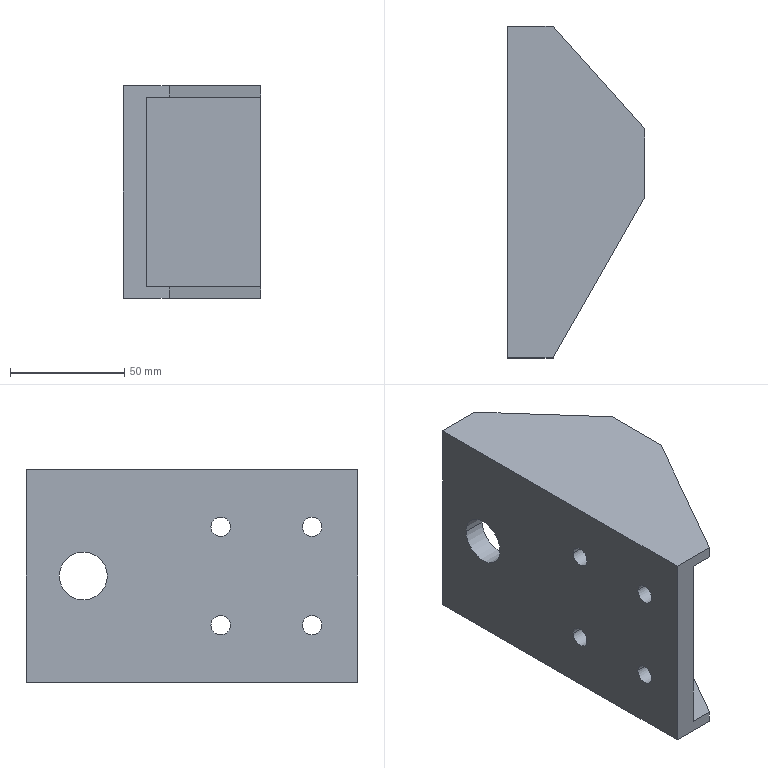Part | NX | features BREP 1 | 1 solid | 28 faces | box 60 x 145 x 93 mm | volume 220117 mm3 | plane 18 | cylinder 10 | commonest cylinder face diameters 8.5 x8 21 x2
STEP:
#1=CARTESIAN_POINT('',(-5.,58.,0.));
#2=VERTEX_POINT('',#1);
#3=CARTESIAN_POINT('',(-5.,37.,0.));
#4=VERTEX_POINT('',#3);
#5=CARTESIAN_POINT('',(-5.,47.5,0.));
#6=DIRECTION('',(-1.,0.,0.));
#7=DIRECTION('',(0.,1.,0.));
#8=AXIS2_PLACEMENT_3D('',#5,#6,#7);
#9=CIRCLE('',#8,10.5);
#10=EDGE_CURVE('',#2,#4,#9,.T.);
#11=ORIENTED_EDGE('',*,*,#10,.T.);
#12=CARTESIAN_POINT('',(5.,37.,0.));
#13=VERTEX_POINT('',#12);
#14=CARTESIAN_POINT('',(-5.,37.,0.));
#15=DIRECTION('',(1.,0.,0.));
#16=VECTOR('',#15,1000.);
#17=LINE('',#14,#16);
#18=EDGE_CURVE('',#13,#4,#17,.F.);
#19=ORIENTED_EDGE('',*,*,#18,.F.);
#20=CARTESIAN_POINT('',(5.,58.,0.));
#21=VERTEX_POINT('',#20);
#22=CARTESIAN_POINT('',(5.,47.5,0.));
#23=DIRECTION('',(-1.,0.,0.));
#24=DIRECTION('',(0.,1.,0.));
#25=AXIS2_PLACEMENT_3D('',#22,#23,#24);
#26=CIRCLE('',#25,10.5);
#27=EDGE_CURVE('',#21,#13,#26,.T.);
#28=ORIENTED_EDGE('',*,*,#27,.F.);
#29=CARTESIAN_POINT('',(-5.,58.,0.));
#30=DIRECTION('',(1.,0.,0.));
#31=VECTOR('',#30,1000.);
#32=LINE('',#29,#31);
#33=EDGE_CURVE('',#21,#2,#32,.F.);
#34=ORIENTED_EDGE('',*,*,#33,.T.);
#35=EDGE_LOOP('',(#11,#19,#28,#34));
#36=FACE_BOUND('',#35,.T.);
#37=CARTESIAN_POINT('',(-5.,47.5,0.));
#38=DIRECTION('',(1.,0.,0.));
#39=DIRECTION('',(0.,1.,0.));
#40=AXIS2_PLACEMENT_3D('',#37,#38,#39);
#41=CYLINDRICAL_SURFACE('',#40,10.5);
#42=ADVANCED_FACE('',(#36),#41,.F.);
#43=CARTESIAN_POINT('',(-5.,-8.25,21.5));
#44=VERTEX_POINT('',#43);
#45=CARTESIAN_POINT('',(-5.,-16.75,21.5));
#46=VERTEX_POINT('',#45);
#47=CARTESIAN_POINT('',(-5.,-12.5,21.5));
#48=DIRECTION('',(-1.,0.,0.));
#49=DIRECTION('',(0.,1.,0.));
#50=AXIS2_PLACEMENT_3D('',#47,#48,#49);
#51=CIRCLE('',#50,4.25);
#52=EDGE_CURVE('',#44,#46,#51,.T.);
#53=ORIENTED_EDGE('',*,*,#52,.T.);
#54=CARTESIAN_POINT('',(5.,-16.75,21.5));
#55=VERTEX_POINT('',#54);
#56=CARTESIAN_POINT('',(-5.,-16.75,21.5));
#57=DIRECTION('',(1.,0.,0.));
#58=VECTOR('',#57,1000.);
#59=LINE('',#56,#58);
#60=EDGE_CURVE('',#55,#46,#59,.F.);
#61=ORIENTED_EDGE('',*,*,#60,.F.);
#62=CARTESIAN_POINT('',(5.,-8.25,21.5));
#63=VERTEX_POINT('',#62);
#64=CARTESIAN_POINT('',(5.,-12.5,21.5));
#65=DIRECTION('',(-1.,0.,0.));
#66=DIRECTION('',(0.,1.,0.));
#67=AXIS2_PLACEMENT_3D('',#64,#65,#66);
#68=CIRCLE('',#67,4.25);
#69=EDGE_CURVE('',#63,#55,#68,.T.);
#70=ORIENTED_EDGE('',*,*,#69,.F.);
#71=CARTESIAN_POINT('',(-5.,-8.25,21.5));
#72=DIRECTION('',(1.,0.,0.));
#73=VECTOR('',#72,1000.);
#74=LINE('',#71,#73);
#75=EDGE_CURVE('',#63,#44,#74,.F.);
#76=ORIENTED_EDGE('',*,*,#75,.T.);
#77=EDGE_LOOP('',(#53,#61,#70,#76));
#78=FACE_BOUND('',#77,.T.);
#79=CARTESIAN_POINT('',(-5.,-12.5,21.5));
#80=DIRECTION('',(1.,0.,0.));
#81=DIRECTION('',(0.,1.,0.));
#82=AXIS2_PLACEMENT_3D('',#79,#80,#81);
#83=CYLINDRICAL_SURFACE('',#82,4.25);
#84=ADVANCED_FACE('',(#78),#83,.F.);
#85=CARTESIAN_POINT('',(-5.,-8.25,-21.5));
#86=VERTEX_POINT('',#85);
#87=CARTESIAN_POINT('',(-5.,-16.75,-21.5));
#88=VERTEX_POINT('',#87);
#89=CARTESIAN_POINT('',(-5.,-12.5,-21.5));
#90=DIRECTION('',(-1.,0.,0.));
#91=DIRECTION('',(0.,1.,0.));
#92=AXIS2_PLACEMENT_3D('',#89,#90,#91);
#93=CIRCLE('',#92,4.25);
#94=EDGE_CURVE('',#86,#88,#93,.T.);
#95=ORIENTED_EDGE('',*,*,#94,.T.);
#96=CARTESIAN_POINT('',(5.,-16.75,-21.5));
#97=VERTEX_POINT('',#96);
#98=CARTESIAN_POINT('',(-5.,-16.75,-21.5));
#99=DIRECTION('',(1.,0.,0.));
#100=VECTOR('',#99,1000.);
#101=LINE('',#98,#100);
#102=EDGE_CURVE('',#97,#88,#101,.F.);
#103=ORIENTED_EDGE('',*,*,#102,.F.);
#104=CARTESIAN_POINT('',(5.,-8.25,-21.5));
#105=VERTEX_POINT('',#104);
#106=CARTESIAN_POINT('',(5.,-12.5,-21.5));
#107=DIRECTION('',(-1.,0.,0.));
#108=DIRECTION('',(0.,1.,0.));
#109=AXIS2_PLACEMENT_3D('',#106,#107,#108);
#110=CIRCLE('',#109,4.25);
#111=EDGE_CURVE('',#105,#97,#110,.T.);
#112=ORIENTED_EDGE('',*,*,#111,.F.);
#113=CARTESIAN_POINT('',(-5.,-8.25,-21.5));
#114=DIRECTION('',(1.,0.,0.));
#115=VECTOR('',#114,1000.);
#116=LINE('',#113,#115);
#117=EDGE_CURVE('',#105,#86,#116,.F.);
#118=ORIENTED_EDGE('',*,*,#117,.T.);
#119=EDGE_LOOP('',(#95,#103,#112,#118));
#120=FACE_BOUND('',#119,.T.);
#121=CARTESIAN_POINT('',(-5.,-12.5,-21.5));
#122=DIRECTION('',(1.,0.,0.));
#123=DIRECTION('',(0.,1.,0.));
#124=AXIS2_PLACEMENT_3D('',#121,#122,#123);
#125=CYLINDRICAL_SURFACE('',#124,4.25);
#126=ADVANCED_FACE('',(#120),#125,.F.);
#127=CARTESIAN_POINT('',(-5.,-48.25,-21.5));
#128=VERTEX_POINT('',#127);
#129=CARTESIAN_POINT('',(-5.,-56.75,-21.5));
#130=VERTEX_POINT('',#129);
#131=CARTESIAN_POINT('',(-5.,-52.5,-21.5));
#132=DIRECTION('',(-1.,0.,0.));
#133=DIRECTION('',(0.,1.,0.));
#134=AXIS2_PLACEMENT_3D('',#131,#132,#133);
#135=CIRCLE('',#134,4.25);
#136=EDGE_CURVE('',#128,#130,#135,.T.);
#137=ORIENTED_EDGE('',*,*,#136,.T.);
#138=CARTESIAN_POINT('',(5.,-56.75,-21.5));
#139=VERTEX_POINT('',#138);
#140=CARTESIAN_POINT('',(-5.,-56.75,-21.5));
#141=DIRECTION('',(1.,0.,0.));
#142=VECTOR('',#141,1000.);
#143=LINE('',#140,#142);
#144=EDGE_CURVE('',#139,#130,#143,.F.);
#145=ORIENTED_EDGE('',*,*,#144,.F.);
#146=CARTESIAN_POINT('',(5.,-48.25,-21.5));
#147=VERTEX_POINT('',#146);
#148=CARTESIAN_POINT('',(5.,-52.5,-21.5));
#149=DIRECTION('',(-1.,0.,0.));
#150=DIRECTION('',(0.,1.,0.));
#151=AXIS2_PLACEMENT_3D('',#148,#149,#150);
#152=CIRCLE('',#151,4.25);
#153=EDGE_CURVE('',#147,#139,#152,.T.);
#154=ORIENTED_EDGE('',*,*,#153,.F.);
#155=CARTESIAN_POINT('',(-5.,-48.25,-21.5));
#156=DIRECTION('',(1.,0.,0.));
#157=VECTOR('',#156,1000.);
#158=LINE('',#155,#157);
#159=EDGE_CURVE('',#147,#128,#158,.F.);
#160=ORIENTED_EDGE('',*,*,#159,.T.);
#161=EDGE_LOOP('',(#137,#145,#154,#160));
#162=FACE_BOUND('',#161,.T.);
#163=CARTESIAN_POINT('',(-5.,-52.5,-21.5));
#164=DIRECTION('',(1.,0.,0.));
#165=DIRECTION('',(0.,1.,0.));
#166=AXIS2_PLACEMENT_3D('',#163,#164,#165);
#167=CYLINDRICAL_SURFACE('',#166,4.25);
#168=ADVANCED_FACE('',(#162),#167,.F.);
#169=CARTESIAN_POINT('',(-5.,-48.25,21.5));
#170=VERTEX_POINT('',#169);
#171=CARTESIAN_POINT('',(-5.,-56.75,21.5));
#172=VERTEX_POINT('',#171);
#173=CARTESIAN_POINT('',(-5.,-52.5,21.5));
#174=DIRECTION('',(-1.,0.,0.));
#175=DIRECTION('',(0.,1.,0.));
#176=AXIS2_PLACEMENT_3D('',#173,#174,#175);
#177=CIRCLE('',#176,4.25);
#178=EDGE_CURVE('',#170,#172,#177,.T.);
#179=ORIENTED_EDGE('',*,*,#178,.T.);
#180=CARTESIAN_POINT('',(5.,-56.75,21.5));
#181=VERTEX_POINT('',#180);
#182=CARTESIAN_POINT('',(-5.,-56.75,21.5));
#183=DIRECTION('',(1.,0.,0.));
#184=VECTOR('',#183,1000.);
#185=LINE('',#182,#184);
#186=EDGE_CURVE('',#181,#172,#185,.F.);
#187=ORIENTED_EDGE('',*,*,#186,.F.);
#188=CARTESIAN_POINT('',(5.,-48.25,21.5));
#189=VERTEX_POINT('',#188);
#190=CARTESIAN_POINT('',(5.,-52.5,21.5));
#191=DIRECTION('',(-1.,0.,0.));
#192=DIRECTION('',(0.,1.,0.));
#193=AXIS2_PLACEMENT_3D('',#190,#191,#192);
#194=CIRCLE('',#193,4.25);
#195=EDGE_CURVE('',#189,#181,#194,.T.);
#196=ORIENTED_EDGE('',*,*,#195,.F.);
#197=CARTESIAN_POINT('',(-5.,-48.25,21.5));
#198=DIRECTION('',(1.,0.,0.));
#199=VECTOR('',#198,1000.);
#200=LINE('',#197,#199);
#201=EDGE_CURVE('',#189,#170,#200,.F.);
#202=ORIENTED_EDGE('',*,*,#201,.T.);
#203=EDGE_LOOP('',(#179,#187,#196,#202));
#204=FACE_BOUND('',#203,.T.);
#205=CARTESIAN_POINT('',(-5.,-52.5,21.5));
#206=DIRECTION('',(1.,0.,0.));
#207=DIRECTION('',(0.,1.,0.));
#208=AXIS2_PLACEMENT_3D('',#205,#206,#207);
#209=CYLINDRICAL_SURFACE('',#208,4.25);
#210=ADVANCED_FACE('',(#204),#209,.F.);
#211=CARTESIAN_POINT('',(-5.,-72.5,46.5));
#212=VERTEX_POINT('',#211);
#213=CARTESIAN_POINT('',(-5.,-72.5,-46.5));
#214=VERTEX_POINT('',#213);
#215=CARTESIAN_POINT('',(-5.,-72.5,46.5));
#216=DIRECTION('',(0.,0.,-1.));
#217=VECTOR('',#216,1000.);
#218=LINE('',#215,#217);
#219=EDGE_CURVE('',#212,#214,#218,.T.);
#220=ORIENTED_EDGE('',*,*,#219,.F.);
#221=CARTESIAN_POINT('',(-5.,72.5,46.5));
#222=VERTEX_POINT('',#221);
#223=CARTESIAN_POINT('',(-5.,72.5,46.5));
#224=DIRECTION('',(0.,-1.,0.));
#225=VECTOR('',#224,1000.);
#226=LINE('',#223,#225);
#227=EDGE_CURVE('',#222,#212,#226,.T.);
#228=ORIENTED_EDGE('',*,*,#227,.F.);
#229=CARTESIAN_POINT('',(-5.,72.5,-46.5));
#230=VERTEX_POINT('',#229);
#231=CARTESIAN_POINT('',(-5.,72.5,46.5));
#232=DIRECTION('',(0.,0.,1.));
#233=VECTOR('',#232,1000.);
#234=LINE('',#231,#233);
#235=EDGE_CURVE('',#230,#222,#234,.T.);
#236=ORIENTED_EDGE('',*,*,#235,.F.);
#237=CARTESIAN_POINT('',(-5.,72.5,-46.5));
#238=DIRECTION('',(0.,1.,0.));
#239=VECTOR('',#238,1000.);
#240=LINE('',#237,#239);
#241=EDGE_CURVE('',#214,#230,#240,.T.);
#242=ORIENTED_EDGE('',*,*,#241,.F.);
#243=EDGE_LOOP('',(#220,#228,#236,#242));
#244=FACE_BOUND('',#243,.T.);
#245=ORIENTED_EDGE('',*,*,#10,.F.);
#246=CARTESIAN_POINT('',(-5.,47.5,0.));
#247=DIRECTION('',(-1.,0.,0.));
#248=DIRECTION('',(0.,1.,0.));
#249=AXIS2_PLACEMENT_3D('',#246,#247,#248);
#250=CIRCLE('',#249,10.5);
#251=EDGE_CURVE('',#4,#2,#250,.T.);
#252=ORIENTED_EDGE('',*,*,#251,.F.);
#253=EDGE_LOOP('',(#245,#252));
#254=FACE_BOUND('',#253,.T.);
#255=ORIENTED_EDGE('',*,*,#52,.F.);
#256=CARTESIAN_POINT('',(-5.,-12.5,21.5));
#257=DIRECTION('',(-1.,0.,0.));
#258=DIRECTION('',(0.,1.,0.));
#259=AXIS2_PLACEMENT_3D('',#256,#257,#258);
#260=CIRCLE('',#259,4.25);
#261=EDGE_CURVE('',#46,#44,#260,.T.);
#262=ORIENTED_EDGE('',*,*,#261,.F.);
#263=EDGE_LOOP('',(#255,#262));
#264=FACE_BOUND('',#263,.T.);
#265=ORIENTED_EDGE('',*,*,#94,.F.);
#266=CARTESIAN_POINT('',(-5.,-12.5,-21.5));
#267=DIRECTION('',(-1.,0.,0.));
#268=DIRECTION('',(0.,1.,0.));
#269=AXIS2_PLACEMENT_3D('',#266,#267,#268);
#270=CIRCLE('',#269,4.25);
#271=EDGE_CURVE('',#88,#86,#270,.T.);
#272=ORIENTED_EDGE('',*,*,#271,.F.);
#273=EDGE_LOOP('',(#265,#272));
#274=FACE_BOUND('',#273,.T.);
#275=ORIENTED_EDGE('',*,*,#136,.F.);
#276=CARTESIAN_POINT('',(-5.,-52.5,-21.5));
#277=DIRECTION('',(-1.,0.,0.));
#278=DIRECTION('',(0.,1.,0.));
#279=AXIS2_PLACEMENT_3D('',#276,#277,#278);
#280=CIRCLE('',#279,4.25);
#281=EDGE_CURVE('',#130,#128,#280,.T.);
#282=ORIENTED_EDGE('',*,*,#281,.F.);
#283=EDGE_LOOP('',(#275,#282));
#284=FACE_BOUND('',#283,.T.);
#285=ORIENTED_EDGE('',*,*,#178,.F.);
#286=CARTESIAN_POINT('',(-5.,-52.5,21.5));
#287=DIRECTION('',(-1.,0.,0.));
#288=DIRECTION('',(0.,1.,0.));
#289=AXIS2_PLACEMENT_3D('',#286,#287,#288);
#290=CIRCLE('',#289,4.25);
#291=EDGE_CURVE('',#172,#170,#290,.T.);
#292=ORIENTED_EDGE('',*,*,#291,.F.);
#293=EDGE_LOOP('',(#285,#292));
#294=FACE_BOUND('',#293,.T.);
#295=CARTESIAN_POINT('',(-5.,72.5,46.5));
#296=DIRECTION('',(1.,0.,0.));
#297=DIRECTION('',(0.,1.,0.));
#298=AXIS2_PLACEMENT_3D('',#295,#296,#297);
#299=PLANE('',#298);
#300=ADVANCED_FACE('',(#244,#254,#264,#274,#284,#294),#299,.F.);
#301=CARTESIAN_POINT('',(55.,-2.5,-46.5));
#302=VERTEX_POINT('',#301);
#303=CARTESIAN_POINT('',(55.,27.5,-46.5));
#304=VERTEX_POINT('',#303);
#305=CARTESIAN_POINT('',(55.,-72.5,-46.5));
#306=DIRECTION('',(0.,1.,0.));
#307=VECTOR('',#306,1000.);
#308=LINE('',#305,#307);
#309=EDGE_CURVE('',#302,#304,#308,.T.);
#310=ORIENTED_EDGE('',*,*,#309,.F.);
#311=CARTESIAN_POINT('',(15.,-72.5,-46.5));
#312=VERTEX_POINT('',#311);
#313=CARTESIAN_POINT('',(15.,-72.5,-46.5));
#314=DIRECTION('',(0.4961,0.8682,0.));
#315=VECTOR('',#314,1000.);
#316=LINE('',#313,#315);
#317=EDGE_CURVE('',#312,#302,#316,.T.);
#318=ORIENTED_EDGE('',*,*,#317,.F.);
#319=CARTESIAN_POINT('',(5.,-72.5,-46.5));
#320=DIRECTION('',(1.,0.,0.));
#321=VECTOR('',#320,1000.);
#322=LINE('',#319,#321);
#323=EDGE_CURVE('',#214,#312,#322,.T.);
#324=ORIENTED_EDGE('',*,*,#323,.F.);
#325=ORIENTED_EDGE('',*,*,#241,.T.);
#326=CARTESIAN_POINT('',(15.,72.5,-46.5));
#327=VERTEX_POINT('',#326);
#328=CARTESIAN_POINT('',(5.,72.5,-46.5));
#329=DIRECTION('',(-1.,0.,0.));
#330=VECTOR('',#329,1000.);
#331=LINE('',#328,#330);
#332=EDGE_CURVE('',#327,#230,#331,.T.);
#333=ORIENTED_EDGE('',*,*,#332,.F.);
#334=CARTESIAN_POINT('',(55.,27.5,-46.5));
#335=DIRECTION('',(-0.6644,0.7474,0.));
#336=VECTOR('',#335,1000.);
#337=LINE('',#334,#336);
#338=EDGE_CURVE('',#304,#327,#337,.T.);
#339=ORIENTED_EDGE('',*,*,#338,.F.);
#340=EDGE_LOOP('',(#310,#318,#324,#325,#333,#339));
#341=FACE_BOUND('',#340,.T.);
#342=CARTESIAN_POINT('',(5.,-72.5,-46.5));
#343=DIRECTION('',(0.,0.,1.));
#344=DIRECTION('',(1.,0.,0.));
#345=AXIS2_PLACEMENT_3D('',#342,#343,#344);
#346=PLANE('',#345);
#347=ADVANCED_FACE('',(#341),#346,.F.);
#348=CARTESIAN_POINT('',(15.,-72.5,-41.5));
#349=VERTEX_POINT('',#348);
#350=CARTESIAN_POINT('',(15.,-72.5,46.5));
#351=DIRECTION('',(0.,0.,-1.));
#352=VECTOR('',#351,1000.);
#353=LINE('',#350,#352);
#354=EDGE_CURVE('',#349,#312,#353,.T.);
#355=ORIENTED_EDGE('',*,*,#354,.F.);
#356=CARTESIAN_POINT('',(5.,-72.5,-41.5));
#357=VERTEX_POINT('',#356);
#358=CARTESIAN_POINT('',(-5.,-72.5,-41.5));
#359=DIRECTION('',(1.,0.,0.));
#360=VECTOR('',#359,1000.);
#361=LINE('',#358,#360);
#362=EDGE_CURVE('',#357,#349,#361,.T.);
#363=ORIENTED_EDGE('',*,*,#362,.F.);
#364=CARTESIAN_POINT('',(5.,-72.5,41.5));
#365=VERTEX_POINT('',#364);
#366=CARTESIAN_POINT('',(5.,-72.5,46.5));
#367=DIRECTION('',(0.,0.,-1.));
#368=VECTOR('',#367,1000.);
#369=LINE('',#366,#368);
#370=EDGE_CURVE('',#365,#357,#369,.T.);
#371=ORIENTED_EDGE('',*,*,#370,.F.);
#372=CARTESIAN_POINT('',(15.,-72.5,41.5));
#373=VERTEX_POINT('',#372);
#374=CARTESIAN_POINT('',(-5.,-72.5,41.5));
#375=DIRECTION('',(-1.,0.,0.));
#376=VECTOR('',#375,1000.);
#377=LINE('',#374,#376);
#378=EDGE_CURVE('',#373,#365,#377,.T.);
#379=ORIENTED_EDGE('',*,*,#378,.F.);
#380=CARTESIAN_POINT('',(15.,-72.5,46.5));
#381=VERTEX_POINT('',#380);
#382=CARTESIAN_POINT('',(15.,-72.5,46.5));
#383=DIRECTION('',(0.,0.,-1.));
#384=VECTOR('',#383,1000.);
#385=LINE('',#382,#384);
#386=EDGE_CURVE('',#381,#373,#385,.T.);
#387=ORIENTED_EDGE('',*,*,#386,.F.);
#388=CARTESIAN_POINT('',(-5.,-72.5,46.5));
#389=DIRECTION('',(1.,0.,0.));
#390=VECTOR('',#389,1000.);
#391=LINE('',#388,#390);
#392=EDGE_CURVE('',#212,#381,#391,.T.);
#393=ORIENTED_EDGE('',*,*,#392,.F.);
#394=ORIENTED_EDGE('',*,*,#219,.T.);
#395=ORIENTED_EDGE('',*,*,#323,.T.);
#396=EDGE_LOOP('',(#355,#363,#371,#379,#387,#393,#394,#395));
#397=FACE_BOUND('',#396,.T.);
#398=CARTESIAN_POINT('',(-5.,-72.5,46.5));
#399=DIRECTION('',(0.,1.,0.));
#400=DIRECTION('',(1.,0.,0.));
#401=AXIS2_PLACEMENT_3D('',#398,#399,#400);
#402=PLANE('',#401);
#403=ADVANCED_FACE('',(#397),#402,.F.);
#404=CARTESIAN_POINT('',(55.,-2.5,46.5));
#405=VERTEX_POINT('',#404);
#406=CARTESIAN_POINT('',(15.,-72.5,46.5));
#407=DIRECTION('',(0.4961,0.8682,0.));
#408=VECTOR('',#407,1000.);
#409=LINE('',#406,#408);
#410=EDGE_CURVE('',#381,#405,#409,.T.);
#411=ORIENTED_EDGE('',*,*,#410,.T.);
#412=CARTESIAN_POINT('',(55.,27.5,46.5));
#413=VERTEX_POINT('',#412);
#414=CARTESIAN_POINT('',(55.,-72.5,46.5));
#415=DIRECTION('',(0.,1.,0.));
#416=VECTOR('',#415,1000.);
#417=LINE('',#414,#416);
#418=EDGE_CURVE('',#405,#413,#417,.T.);
#419=ORIENTED_EDGE('',*,*,#418,.T.);
#420=CARTESIAN_POINT('',(15.,72.5,46.5));
#421=VERTEX_POINT('',#420);
#422=CARTESIAN_POINT('',(55.,27.5,46.5));
#423=DIRECTION('',(-0.6644,0.7474,0.));
#424=VECTOR('',#423,1000.);
#425=LINE('',#422,#424);
#426=EDGE_CURVE('',#413,#421,#425,.T.);
#427=ORIENTED_EDGE('',*,*,#426,.T.);
#428=CARTESIAN_POINT('',(5.,72.5,46.5));
#429=DIRECTION('',(-1.,0.,0.));
#430=VECTOR('',#429,1000.);
#431=LINE('',#428,#430);
#432=EDGE_CURVE('',#421,#222,#431,.T.);
#433=ORIENTED_EDGE('',*,*,#432,.T.);
#434=ORIENTED_EDGE('',*,*,#227,.T.);
#435=ORIENTED_EDGE('',*,*,#392,.T.);
#436=EDGE_LOOP('',(#411,#419,#427,#433,#434,#435));
#437=FACE_BOUND('',#436,.T.);
#438=CARTESIAN_POINT('',(5.,-72.5,46.5));
#439=DIRECTION('',(0.,0.,1.));
#440=DIRECTION('',(1.,0.,0.));
#441=AXIS2_PLACEMENT_3D('',#438,#439,#440);
#442=PLANE('',#441);
#443=ADVANCED_FACE('',(#437),#442,.T.);
#444=ORIENTED_EDGE('',*,*,#235,.T.);
#445=ORIENTED_EDGE('',*,*,#432,.F.);
#446=CARTESIAN_POINT('',(15.,72.5,41.5));
#447=VERTEX_POINT('',#446);
#448=CARTESIAN_POINT('',(15.,72.5,46.5));
#449=DIRECTION('',(0.,0.,1.));
#450=VECTOR('',#449,1000.);
#451=LINE('',#448,#450);
#452=EDGE_CURVE('',#447,#421,#451,.T.);
#453=ORIENTED_EDGE('',*,*,#452,.F.);
#454=CARTESIAN_POINT('',(5.,72.5,41.5));
#455=VERTEX_POINT('',#454);
#456=CARTESIAN_POINT('',(-5.,72.5,41.5));
#457=DIRECTION('',(1.,0.,0.));
#458=VECTOR('',#457,1000.);
#459=LINE('',#456,#458);
#460=EDGE_CURVE('',#455,#447,#459,.T.);
#461=ORIENTED_EDGE('',*,*,#460,.F.);
#462=CARTESIAN_POINT('',(5.,72.5,-41.5));
#463=VERTEX_POINT('',#462);
#464=CARTESIAN_POINT('',(5.,72.5,46.5));
#465=DIRECTION('',(0.,0.,1.));
#466=VECTOR('',#465,1000.);
#467=LINE('',#464,#466);
#468=EDGE_CURVE('',#463,#455,#467,.T.);
#469=ORIENTED_EDGE('',*,*,#468,.F.);
#470=CARTESIAN_POINT('',(15.,72.5,-41.5));
#471=VERTEX_POINT('',#470);
#472=CARTESIAN_POINT('',(-5.,72.5,-41.5));
#473=DIRECTION('',(-1.,0.,0.));
#474=VECTOR('',#473,1000.);
#475=LINE('',#472,#474);
#476=EDGE_CURVE('',#471,#463,#475,.T.);
#477=ORIENTED_EDGE('',*,*,#476,.F.);
#478=CARTESIAN_POINT('',(15.,72.5,46.5));
#479=DIRECTION('',(0.,0.,1.));
#480=VECTOR('',#479,1000.);
#481=LINE('',#478,#480);
#482=EDGE_CURVE('',#327,#471,#481,.T.);
#483=ORIENTED_EDGE('',*,*,#482,.F.);
#484=ORIENTED_EDGE('',*,*,#332,.T.);
#485=EDGE_LOOP('',(#444,#445,#453,#461,#469,#477,#483,#484));
#486=FACE_BOUND('',#485,.T.);
#487=CARTESIAN_POINT('',(-5.,72.5,46.5));
#488=DIRECTION('',(0.,-1.,0.));
#489=DIRECTION('',(0.,0.,-1.));
#490=AXIS2_PLACEMENT_3D('',#487,#488,#489);
#491=PLANE('',#490);
#492=ADVANCED_FACE('',(#486),#491,.F.);
#493=ORIENTED_EDGE('',*,*,#18,.T.);
#494=ORIENTED_EDGE('',*,*,#251,.T.);
#495=ORIENTED_EDGE('',*,*,#33,.F.);
#496=CARTESIAN_POINT('',(5.,47.5,0.));
#497=DIRECTION('',(-1.,0.,0.));
#498=DIRECTION('',(0.,1.,0.));
#499=AXIS2_PLACEMENT_3D('',#496,#497,#498);
#500=CIRCLE('',#499,10.5);
#501=EDGE_CURVE('',#13,#21,#500,.T.);
#502=ORIENTED_EDGE('',*,*,#501,.F.);
#503=EDGE_LOOP('',(#493,#494,#495,#502));
#504=FACE_BOUND('',#503,.T.);
#505=CARTESIAN_POINT('',(-5.,47.5,0.));
#506=DIRECTION('',(1.,0.,0.));
#507=DIRECTION('',(0.,1.,0.));
#508=AXIS2_PLACEMENT_3D('',#505,#506,#507);
#509=CYLINDRICAL_SURFACE('',#508,10.5);
#510=ADVANCED_FACE('',(#504),#509,.F.);
#511=ORIENTED_EDGE('',*,*,#60,.T.);
#512=ORIENTED_EDGE('',*,*,#261,.T.);
#513=ORIENTED_EDGE('',*,*,#75,.F.);
#514=CARTESIAN_POINT('',(5.,-12.5,21.5));
#515=DIRECTION('',(-1.,0.,0.));
#516=DIRECTION('',(0.,1.,0.));
#517=AXIS2_PLACEMENT_3D('',#514,#515,#516);
#518=CIRCLE('',#517,4.25);
#519=EDGE_CURVE('',#55,#63,#518,.T.);
#520=ORIENTED_EDGE('',*,*,#519,.F.);
#521=EDGE_LOOP('',(#511,#512,#513,#520));
#522=FACE_BOUND('',#521,.T.);
#523=CARTESIAN_POINT('',(-5.,-12.5,21.5));
#524=DIRECTION('',(1.,0.,0.));
#525=DIRECTION('',(0.,1.,0.));
#526=AXIS2_PLACEMENT_3D('',#523,#524,#525);
#527=CYLINDRICAL_SURFACE('',#526,4.25);
#528=ADVANCED_FACE('',(#522),#527,.F.);
#529=ORIENTED_EDGE('',*,*,#102,.T.);
#530=ORIENTED_EDGE('',*,*,#271,.T.);
#531=ORIENTED_EDGE('',*,*,#117,.F.);
#532=CARTESIAN_POINT('',(5.,-12.5,-21.5));
#533=DIRECTION('',(-1.,0.,0.));
#534=DIRECTION('',(0.,1.,0.));
#535=AXIS2_PLACEMENT_3D('',#532,#533,#534);
#536=CIRCLE('',#535,4.25);
#537=EDGE_CURVE('',#97,#105,#536,.T.);
#538=ORIENTED_EDGE('',*,*,#537,.F.);
#539=EDGE_LOOP('',(#529,#530,#531,#538));
#540=FACE_BOUND('',#539,.T.);
#541=CARTESIAN_POINT('',(-5.,-12.5,-21.5));
#542=DIRECTION('',(1.,0.,0.));
#543=DIRECTION('',(0.,1.,0.));
#544=AXIS2_PLACEMENT_3D('',#541,#542,#543);
#545=CYLINDRICAL_SURFACE('',#544,4.25);
#546=ADVANCED_FACE('',(#540),#545,.F.);
#547=ORIENTED_EDGE('',*,*,#144,.T.);
#548=ORIENTED_EDGE('',*,*,#281,.T.);
#549=ORIENTED_EDGE('',*,*,#159,.F.);
#550=CARTESIAN_POINT('',(5.,-52.5,-21.5));
#551=DIRECTION('',(-1.,0.,0.));
#552=DIRECTION('',(0.,1.,0.));
#553=AXIS2_PLACEMENT_3D('',#550,#551,#552);
#554=CIRCLE('',#553,4.25);
#555=EDGE_CURVE('',#139,#147,#554,.T.);
#556=ORIENTED_EDGE('',*,*,#555,.F.);
#557=EDGE_LOOP('',(#547,#548,#549,#556));
#558=FACE_BOUND('',#557,.T.);
#559=CARTESIAN_POINT('',(-5.,-52.5,-21.5));
#560=DIRECTION('',(1.,0.,0.));
#561=DIRECTION('',(0.,1.,0.));
#562=AXIS2_PLACEMENT_3D('',#559,#560,#561);
#563=CYLINDRICAL_SURFACE('',#562,4.25);
#564=ADVANCED_FACE('',(#558),#563,.F.);
#565=ORIENTED_EDGE('',*,*,#186,.T.);
#566=ORIENTED_EDGE('',*,*,#291,.T.);
#567=ORIENTED_EDGE('',*,*,#201,.F.);
#568=CARTESIAN_POINT('',(5.,-52.5,21.5));
#569=DIRECTION('',(-1.,0.,0.));
#570=DIRECTION('',(0.,1.,0.));
#571=AXIS2_PLACEMENT_3D('',#568,#569,#570);
#572=CIRCLE('',#571,4.25);
#573=EDGE_CURVE('',#181,#189,#572,.T.);
#574=ORIENTED_EDGE('',*,*,#573,.F.);
#575=EDGE_LOOP('',(#565,#566,#567,#574));
#576=FACE_BOUND('',#575,.T.);
#577=CARTESIAN_POINT('',(-5.,-52.5,21.5));
#578=DIRECTION('',(1.,0.,0.));
#579=DIRECTION('',(0.,1.,0.));
#580=AXIS2_PLACEMENT_3D('',#577,#578,#579);
#581=CYLINDRICAL_SURFACE('',#580,4.25);
#582=ADVANCED_FACE('',(#576),#581,.F.);
#583=ORIENTED_EDGE('',*,*,#338,.T.);
#584=ORIENTED_EDGE('',*,*,#482,.T.);
#585=CARTESIAN_POINT('',(55.,27.5,-41.5));
#586=VERTEX_POINT('',#585);
#587=CARTESIAN_POINT('',(55.,27.5,-41.5));
#588=DIRECTION('',(0.6644,-0.7474,0.));
#589=VECTOR('',#588,1000.);
#590=LINE('',#587,#589);
#591=EDGE_CURVE('',#471,#586,#590,.T.);
#592=ORIENTED_EDGE('',*,*,#591,.T.);
#593=CARTESIAN_POINT('',(55.,27.5,-46.5));
#594=DIRECTION('',(0.,0.,-1.));
#595=VECTOR('',#594,1000.);
#596=LINE('',#593,#595);
#597=EDGE_CURVE('',#586,#304,#596,.T.);
#598=ORIENTED_EDGE('',*,*,#597,.T.);
#599=EDGE_LOOP('',(#583,#584,#592,#598));
#600=FACE_BOUND('',#599,.T.);
#601=CARTESIAN_POINT('',(55.,27.5,-46.5));
#602=DIRECTION('',(0.7474,0.6644,0.));
#603=DIRECTION('',(0.,0.,-1.));
#604=AXIS2_PLACEMENT_3D('',#601,#602,#603);
#605=PLANE('',#604);
#606=ADVANCED_FACE('',(#600),#605,.T.);
#607=CARTESIAN_POINT('',(55.,7.5,-41.5));
#608=VERTEX_POINT('',#607);
#609=CARTESIAN_POINT('',(55.,-2.5,-41.5));
#610=VERTEX_POINT('',#609);
#611=CARTESIAN_POINT('',(55.,17.5,-41.5));
#612=DIRECTION('',(0.,-1.,0.));
#613=VECTOR('',#612,1000.);
#614=LINE('',#611,#613);
#615=EDGE_CURVE('',#608,#610,#614,.T.);
#616=ORIENTED_EDGE('',*,*,#615,.T.);
#617=CARTESIAN_POINT('',(55.,-2.5,-97.49));
#618=DIRECTION('',(0.,0.,-1.));
#619=VECTOR('',#618,1000.);
#620=LINE('',#617,#619);
#621=EDGE_CURVE('',#610,#302,#620,.T.);
#622=ORIENTED_EDGE('',*,*,#621,.T.);
#623=ORIENTED_EDGE('',*,*,#309,.T.);
#624=ORIENTED_EDGE('',*,*,#597,.F.);
#625=CARTESIAN_POINT('',(55.,17.5,-41.5));
#626=VERTEX_POINT('',#625);
#627=CARTESIAN_POINT('',(55.,17.5,-41.5));
#628=DIRECTION('',(0.,-1.,0.));
#629=VECTOR('',#628,1000.);
#630=LINE('',#627,#629);
#631=EDGE_CURVE('',#586,#626,#630,.T.);
#632=ORIENTED_EDGE('',*,*,#631,.T.);
#633=CARTESIAN_POINT('',(55.,17.5,41.5));
#634=VERTEX_POINT('',#633);
#635=CARTESIAN_POINT('',(55.,17.5,-97.49));
#636=DIRECTION('',(0.,0.,1.));
#637=VECTOR('',#636,1000.);
#638=LINE('',#635,#637);
#639=EDGE_CURVE('',#626,#634,#638,.T.);
#640=ORIENTED_EDGE('',*,*,#639,.T.);
#641=CARTESIAN_POINT('',(55.,27.5,41.5));
#642=VERTEX_POINT('',#641);
#643=CARTESIAN_POINT('',(55.,17.5,41.5));
#644=DIRECTION('',(0.,1.,0.));
#645=VECTOR('',#644,1000.);
#646=LINE('',#643,#645);
#647=EDGE_CURVE('',#634,#642,#646,.T.);
#648=ORIENTED_EDGE('',*,*,#647,.T.);
#649=CARTESIAN_POINT('',(55.,27.5,-97.49));
#650=DIRECTION('',(0.,0.,1.));
#651=VECTOR('',#650,1000.);
#652=LINE('',#649,#651);
#653=EDGE_CURVE('',#642,#413,#652,.T.);
#654=ORIENTED_EDGE('',*,*,#653,.T.);
#655=ORIENTED_EDGE('',*,*,#418,.F.);
#656=CARTESIAN_POINT('',(55.,-2.5,41.5));
#657=VERTEX_POINT('',#656);
#658=CARTESIAN_POINT('',(55.,-2.5,-97.49));
#659=DIRECTION('',(0.,0.,-1.));
#660=VECTOR('',#659,1000.);
#661=LINE('',#658,#660);
#662=EDGE_CURVE('',#405,#657,#661,.T.);
#663=ORIENTED_EDGE('',*,*,#662,.T.);
#664=CARTESIAN_POINT('',(55.,7.5,41.5));
#665=VERTEX_POINT('',#664);
#666=CARTESIAN_POINT('',(55.,17.5,41.5));
#667=DIRECTION('',(0.,1.,0.));
#668=VECTOR('',#667,1000.);
#669=LINE('',#666,#668);
#670=EDGE_CURVE('',#657,#665,#669,.T.);
#671=ORIENTED_EDGE('',*,*,#670,.T.);
#672=CARTESIAN_POINT('',(55.,7.5,-97.49));
#673=DIRECTION('',(0.,0.,-1.));
#674=VECTOR('',#673,1000.);
#675=LINE('',#672,#674);
#676=EDGE_CURVE('',#665,#608,#675,.T.);
#677=ORIENTED_EDGE('',*,*,#676,.T.);
#678=EDGE_LOOP('',(#616,#622,#623,#624,#632,#640,#648,#654,#655,#663,#671,#677));
#679=FACE_BOUND('',#678,.T.);
#680=CARTESIAN_POINT('',(55.,17.5,-97.49));
#681=DIRECTION('',(1.,0.,0.));
#682=DIRECTION('',(0.,1.,0.));
#683=AXIS2_PLACEMENT_3D('',#680,#681,#682);
#684=PLANE('',#683);
#685=ADVANCED_FACE('',(#679),#684,.T.);
#686=ORIENTED_EDGE('',*,*,#317,.T.);
#687=ORIENTED_EDGE('',*,*,#621,.F.);
#688=CARTESIAN_POINT('',(15.,-72.5,-41.5));
#689=DIRECTION('',(-0.4961,-0.8682,0.));
#690=VECTOR('',#689,1000.);
#691=LINE('',#688,#690);
#692=EDGE_CURVE('',#610,#349,#691,.T.);
#693=ORIENTED_EDGE('',*,*,#692,.T.);
#694=ORIENTED_EDGE('',*,*,#354,.T.);
#695=EDGE_LOOP('',(#686,#687,#693,#694));
#696=FACE_BOUND('',#695,.T.);
#697=CARTESIAN_POINT('',(15.,-72.5,-46.5));
#698=DIRECTION('',(0.8682,-0.4961,0.));
#699=DIRECTION('',(0.,0.,-1.));
#700=AXIS2_PLACEMENT_3D('',#697,#698,#699);
#701=PLANE('',#700);
#702=ADVANCED_FACE('',(#696),#701,.T.);
#703=ORIENTED_EDGE('',*,*,#692,.F.);
#704=ORIENTED_EDGE('',*,*,#615,.F.);
#705=CARTESIAN_POINT('',(5.,7.5,-41.5));
#706=VERTEX_POINT('',#705);
#707=CARTESIAN_POINT('',(5.,7.5,-41.5));
#708=DIRECTION('',(-1.,0.,0.));
#709=VECTOR('',#708,1000.);
#710=LINE('',#707,#709);
#711=EDGE_CURVE('',#608,#706,#710,.T.);
#712=ORIENTED_EDGE('',*,*,#711,.T.);
#713=CARTESIAN_POINT('',(5.,7.5,-41.5));
#714=DIRECTION('',(0.,-1.,0.));
#715=VECTOR('',#714,1000.);
#716=LINE('',#713,#715);
#717=EDGE_CURVE('',#706,#357,#716,.T.);
#718=ORIENTED_EDGE('',*,*,#717,.T.);
#719=ORIENTED_EDGE('',*,*,#362,.T.);
#720=EDGE_LOOP('',(#703,#704,#712,#718,#719));
#721=FACE_BOUND('',#720,.T.);
#722=CARTESIAN_POINT('',(5.,7.5,-41.5));
#723=DIRECTION('',(0.,0.,1.));
#724=DIRECTION('',(1.,0.,0.));
#725=AXIS2_PLACEMENT_3D('',#722,#723,#724);
#726=PLANE('',#725);
#727=ADVANCED_FACE('',(#721),#726,.T.);
#728=ORIENTED_EDGE('',*,*,#717,.F.);
#729=CARTESIAN_POINT('',(5.,7.5,41.5));
#730=VERTEX_POINT('',#729);
#731=CARTESIAN_POINT('',(5.,7.5,46.5));
#732=DIRECTION('',(0.,0.,-1.));
#733=VECTOR('',#732,1000.);
#734=LINE('',#731,#733);
#735=EDGE_CURVE('',#730,#706,#734,.T.);
#736=ORIENTED_EDGE('',*,*,#735,.F.);
#737=CARTESIAN_POINT('',(5.,72.5,41.5));
#738=DIRECTION('',(0.,1.,0.));
#739=VECTOR('',#738,1000.);
#740=LINE('',#737,#739);
#741=EDGE_CURVE('',#365,#730,#740,.T.);
#742=ORIENTED_EDGE('',*,*,#741,.F.);
#743=ORIENTED_EDGE('',*,*,#370,.T.);
#744=EDGE_LOOP('',(#728,#736,#742,#743));
#745=FACE_BOUND('',#744,.T.);
#746=ORIENTED_EDGE('',*,*,#69,.T.);
#747=ORIENTED_EDGE('',*,*,#519,.T.);
#748=EDGE_LOOP('',(#746,#747));
#749=FACE_BOUND('',#748,.T.);
#750=ORIENTED_EDGE('',*,*,#111,.T.);
#751=ORIENTED_EDGE('',*,*,#537,.T.);
#752=EDGE_LOOP('',(#750,#751));
#753=FACE_BOUND('',#752,.T.);
#754=ORIENTED_EDGE('',*,*,#153,.T.);
#755=ORIENTED_EDGE('',*,*,#555,.T.);
#756=EDGE_LOOP('',(#754,#755));
#757=FACE_BOUND('',#756,.T.);
#758=ORIENTED_EDGE('',*,*,#195,.T.);
#759=ORIENTED_EDGE('',*,*,#573,.T.);
#760=EDGE_LOOP('',(#758,#759));
#761=FACE_BOUND('',#760,.T.);
#762=CARTESIAN_POINT('',(5.,72.5,46.5));
#763=DIRECTION('',(-1.,0.,0.));
#764=DIRECTION('',(0.,1.,0.));
#765=AXIS2_PLACEMENT_3D('',#762,#763,#764);
#766=PLANE('',#765);
#767=ADVANCED_FACE('',(#745,#749,#753,#757,#761),#766,.F.);
#768=ORIENTED_EDGE('',*,*,#670,.F.);
#769=CARTESIAN_POINT('',(15.,-72.5,41.5));
#770=DIRECTION('',(0.4961,0.8682,0.));
#771=VECTOR('',#770,1000.);
#772=LINE('',#769,#771);
#773=EDGE_CURVE('',#373,#657,#772,.T.);
#774=ORIENTED_EDGE('',*,*,#773,.F.);
#775=ORIENTED_EDGE('',*,*,#378,.T.);
#776=ORIENTED_EDGE('',*,*,#741,.T.);
#777=CARTESIAN_POINT('',(5.,7.5,41.5));
#778=DIRECTION('',(-1.,0.,0.));
#779=VECTOR('',#778,1000.);
#780=LINE('',#777,#779);
#781=EDGE_CURVE('',#665,#730,#780,.T.);
#782=ORIENTED_EDGE('',*,*,#781,.F.);
#783=EDGE_LOOP('',(#768,#774,#775,#776,#782));
#784=FACE_BOUND('',#783,.T.);
#785=CARTESIAN_POINT('',(5.,7.5,41.5));
#786=DIRECTION('',(0.,0.,1.));
#787=DIRECTION('',(1.,0.,0.));
#788=AXIS2_PLACEMENT_3D('',#785,#786,#787);
#789=PLANE('',#788);
#790=ADVANCED_FACE('',(#784),#789,.F.);
#791=ORIENTED_EDGE('',*,*,#773,.T.);
#792=ORIENTED_EDGE('',*,*,#662,.F.);
#793=ORIENTED_EDGE('',*,*,#410,.F.);
#794=ORIENTED_EDGE('',*,*,#386,.T.);
#795=EDGE_LOOP('',(#791,#792,#793,#794));
#796=FACE_BOUND('',#795,.T.);
#797=CARTESIAN_POINT('',(15.,-72.5,41.5));
#798=DIRECTION('',(0.8682,-0.4961,0.));
#799=DIRECTION('',(0.,0.,-1.));
#800=AXIS2_PLACEMENT_3D('',#797,#798,#799);
#801=PLANE('',#800);
#802=ADVANCED_FACE('',(#796),#801,.T.);
#803=CARTESIAN_POINT('',(55.,27.5,41.5));
#804=DIRECTION('',(-0.6644,0.7474,0.));
#805=VECTOR('',#804,1000.);
#806=LINE('',#803,#805);
#807=EDGE_CURVE('',#642,#447,#806,.T.);
#808=ORIENTED_EDGE('',*,*,#807,.T.);
#809=ORIENTED_EDGE('',*,*,#452,.T.);
#810=ORIENTED_EDGE('',*,*,#426,.F.);
#811=ORIENTED_EDGE('',*,*,#653,.F.);
#812=EDGE_LOOP('',(#808,#809,#810,#811));
#813=FACE_BOUND('',#812,.T.);
#814=CARTESIAN_POINT('',(55.,27.5,41.5));
#815=DIRECTION('',(0.7474,0.6644,0.));
#816=DIRECTION('',(0.,0.,-1.));
#817=AXIS2_PLACEMENT_3D('',#814,#815,#816);
#818=PLANE('',#817);
#819=ADVANCED_FACE('',(#813),#818,.T.);
#820=ORIENTED_EDGE('',*,*,#807,.F.);
#821=ORIENTED_EDGE('',*,*,#647,.F.);
#822=CARTESIAN_POINT('',(5.,17.5,41.5));
#823=VERTEX_POINT('',#822);
#824=CARTESIAN_POINT('',(5.,17.5,41.5));
#825=DIRECTION('',(1.,0.,0.));
#826=VECTOR('',#825,1000.);
#827=LINE('',#824,#826);
#828=EDGE_CURVE('',#823,#634,#827,.T.);
#829=ORIENTED_EDGE('',*,*,#828,.F.);
#830=CARTESIAN_POINT('',(5.,72.5,41.5));
#831=DIRECTION('',(0.,-1.,0.));
#832=VECTOR('',#831,1000.);
#833=LINE('',#830,#832);
#834=EDGE_CURVE('',#455,#823,#833,.T.);
#835=ORIENTED_EDGE('',*,*,#834,.F.);
#836=ORIENTED_EDGE('',*,*,#460,.T.);
#837=EDGE_LOOP('',(#820,#821,#829,#835,#836));
#838=FACE_BOUND('',#837,.T.);
#839=CARTESIAN_POINT('',(5.,72.5,41.5));
#840=DIRECTION('',(0.,0.,1.));
#841=DIRECTION('',(1.,0.,0.));
#842=AXIS2_PLACEMENT_3D('',#839,#840,#841);
#843=PLANE('',#842);
#844=ADVANCED_FACE('',(#838),#843,.F.);
#845=CARTESIAN_POINT('',(5.,17.5,-41.5));
#846=VERTEX_POINT('',#845);
#847=CARTESIAN_POINT('',(5.,72.5,-41.5));
#848=DIRECTION('',(0.,-1.,0.));
#849=VECTOR('',#848,1000.);
#850=LINE('',#847,#849);
#851=EDGE_CURVE('',#463,#846,#850,.T.);
#852=ORIENTED_EDGE('',*,*,#851,.F.);
#853=ORIENTED_EDGE('',*,*,#468,.T.);
#854=ORIENTED_EDGE('',*,*,#834,.T.);
#855=CARTESIAN_POINT('',(5.,17.5,46.5));
#856=DIRECTION('',(0.,0.,1.));
#857=VECTOR('',#856,1000.);
#858=LINE('',#855,#857);
#859=EDGE_CURVE('',#846,#823,#858,.T.);
#860=ORIENTED_EDGE('',*,*,#859,.F.);
#861=EDGE_LOOP('',(#852,#853,#854,#860));
#862=FACE_BOUND('',#861,.T.);
#863=ORIENTED_EDGE('',*,*,#27,.T.);
#864=ORIENTED_EDGE('',*,*,#501,.T.);
#865=EDGE_LOOP('',(#863,#864));
#866=FACE_BOUND('',#865,.T.);
#867=CARTESIAN_POINT('',(5.,72.5,46.5));
#868=DIRECTION('',(-1.,0.,0.));
#869=DIRECTION('',(0.,1.,0.));
#870=AXIS2_PLACEMENT_3D('',#867,#868,#869);
#871=PLANE('',#870);
#872=ADVANCED_FACE('',(#862,#866),#871,.F.);
#873=ORIENTED_EDGE('',*,*,#631,.F.);
#874=ORIENTED_EDGE('',*,*,#591,.F.);
#875=ORIENTED_EDGE('',*,*,#476,.T.);
#876=ORIENTED_EDGE('',*,*,#851,.T.);
#877=CARTESIAN_POINT('',(5.,17.5,-41.5));
#878=DIRECTION('',(1.,0.,0.));
#879=VECTOR('',#878,1000.);
#880=LINE('',#877,#879);
#881=EDGE_CURVE('',#846,#626,#880,.T.);
#882=ORIENTED_EDGE('',*,*,#881,.T.);
#883=EDGE_LOOP('',(#873,#874,#875,#876,#882));
#884=FACE_BOUND('',#883,.T.);
#885=CARTESIAN_POINT('',(5.,72.5,-41.5));
#886=DIRECTION('',(0.,0.,1.));
#887=DIRECTION('',(1.,0.,0.));
#888=AXIS2_PLACEMENT_3D('',#885,#886,#887);
#889=PLANE('',#888);
#890=ADVANCED_FACE('',(#884),#889,.T.);
#891=ORIENTED_EDGE('',*,*,#781,.T.);
#892=ORIENTED_EDGE('',*,*,#735,.T.);
#893=ORIENTED_EDGE('',*,*,#711,.F.);
#894=ORIENTED_EDGE('',*,*,#676,.F.);
#895=EDGE_LOOP('',(#891,#892,#893,#894));
#896=FACE_BOUND('',#895,.T.);
#897=CARTESIAN_POINT('',(5.,7.5,-97.49));
#898=DIRECTION('',(0.,-1.,0.));
#899=DIRECTION('',(0.,0.,-1.));
#900=AXIS2_PLACEMENT_3D('',#897,#898,#899);
#901=PLANE('',#900);
#902=ADVANCED_FACE('',(#896),#901,.T.);
#903=ORIENTED_EDGE('',*,*,#828,.T.);
#904=ORIENTED_EDGE('',*,*,#639,.F.);
#905=ORIENTED_EDGE('',*,*,#881,.F.);
#906=ORIENTED_EDGE('',*,*,#859,.T.);
#907=EDGE_LOOP('',(#903,#904,#905,#906));
#908=FACE_BOUND('',#907,.T.);
#909=CARTESIAN_POINT('',(5.,17.5,-97.49));
#910=DIRECTION('',(0.,1.,0.));
#911=DIRECTION('',(1.,0.,0.));
#912=AXIS2_PLACEMENT_3D('',#909,#910,#911);
#913=PLANE('',#912);
#914=ADVANCED_FACE('',(#908),#913,.T.);
#915=CLOSED_SHELL('',(#42,#84,#126,#168,#210,#300,#347,#403,#443,#492,#510,#528,#546,#564,#582,#606,#685,#702,#727,#767,#790,#802,#819,#844,#872,#890,#902,#914));
#916=MANIFOLD_SOLID_BREP('',#915);
#917=(LENGTH_UNIT()NAMED_UNIT(*)SI_UNIT(.MILLI.,.METRE.));
#918=UNCERTAINTY_MEASURE_WITH_UNIT(LENGTH_MEASURE(0.00001),#917,'','');
#919=(NAMED_UNIT(*)PLANE_ANGLE_UNIT()SI_UNIT($,.RADIAN.));
#920=(NAMED_UNIT(*)SI_UNIT($,.STERADIAN.)SOLID_ANGLE_UNIT());
#921=(GEOMETRIC_REPRESENTATION_CONTEXT(3)GLOBAL_UNCERTAINTY_ASSIGNED_CONTEXT((#918))GLOBAL_UNIT_ASSIGNED_CONTEXT((#917,#919,#920))REPRESENTATION_CONTEXT('',''));
#922=ADVANCED_BREP_SHAPE_REPRESENTATION('',(#916),#921);